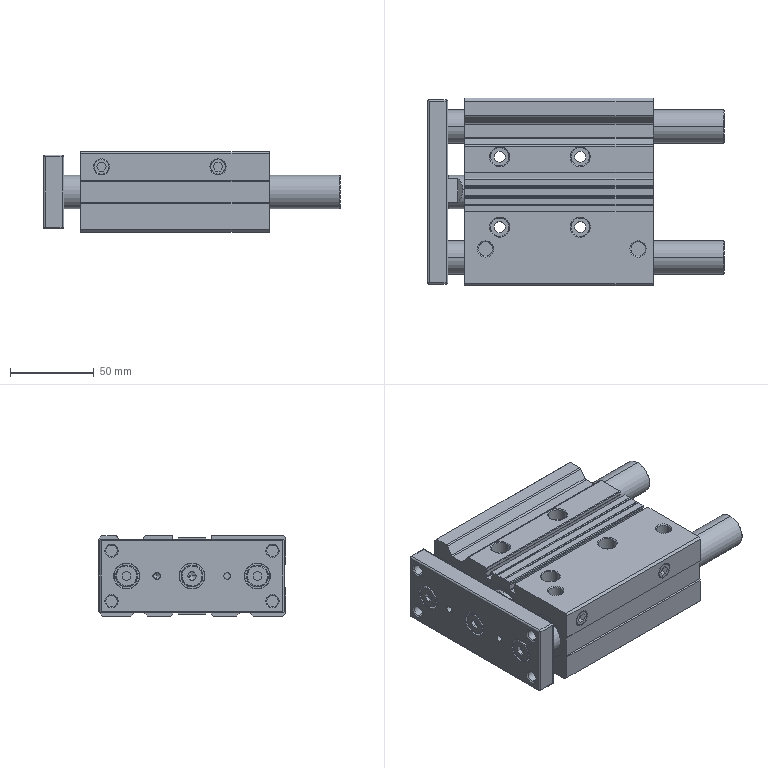Part | SolidWorks | features CompositeCurve 1 | 4 solids | 575 faces | box 177 x 112 x 48 mm | volume 579896 mm3 | cylinder 240 | plane 205 | cone 108 | spline 22 | commonest cylinder face diameters 0.4 x34 0.8 x28 6.647 x26 4 x18 2 x12 20 x12